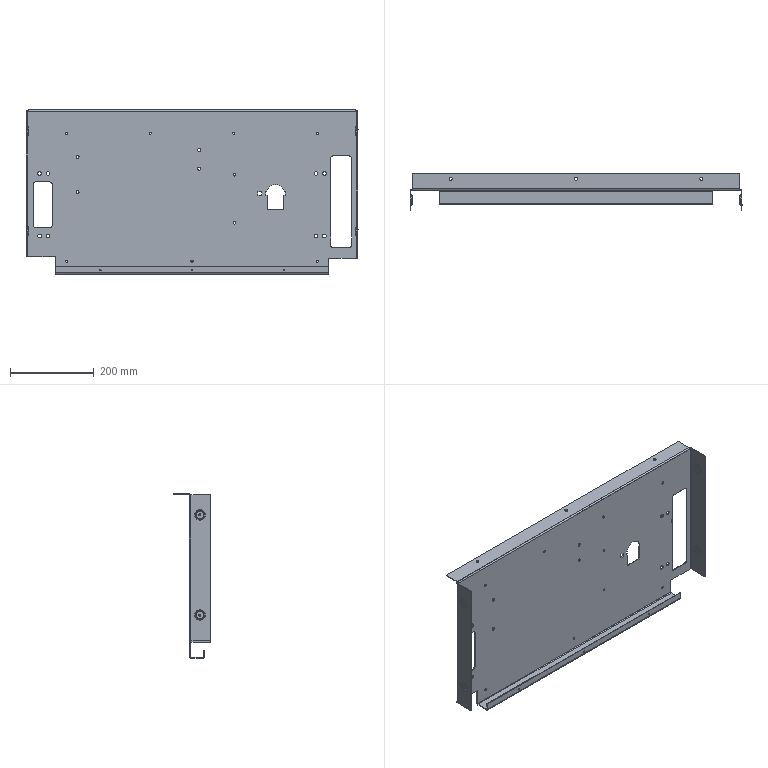Part | STEP file | 1 solid | 203 faces | box 795 x 88 x 393 mm | volume 764007 mm3 | cylinder 98 | plane 73 | torus 32 | commonest cylinder face diameters 7 x19 5.3 x18 9 x16 4.7 x8 13 x8 20 x8